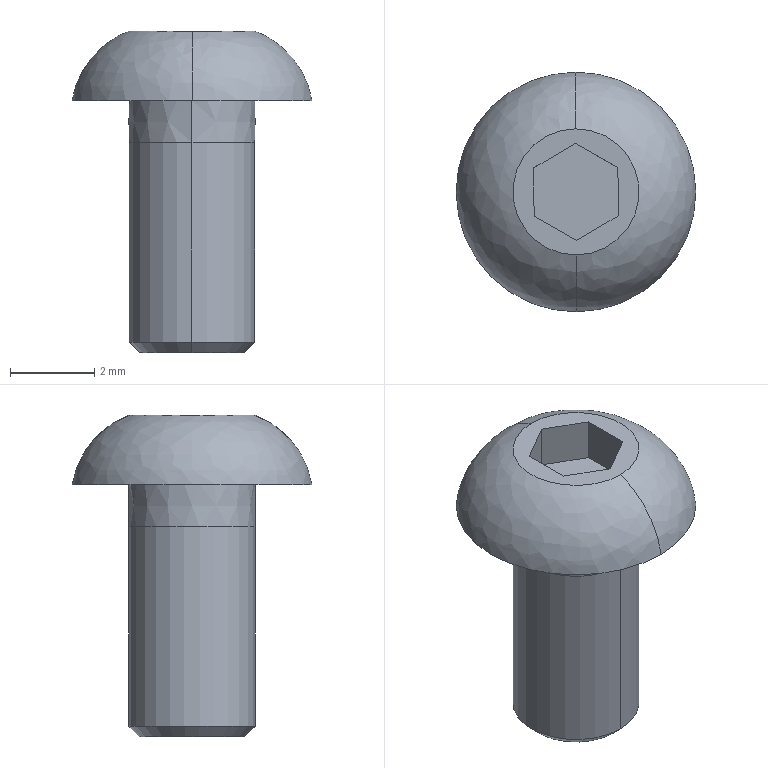Part | SolidWorks | features BaseBody 1 | 1 solid | 18 faces | box 5.7 x 5.7 x 7.65 mm | volume 69.708 mm3 | plane 10 | cone 4 | spline 2 | cylinder 2 | commonest cylinder face diameters 3 x2
STEP:
#1=CARTESIAN_POINT('',(555.46,-174.211,-71.234));
#2=VERTEX_POINT('',#1);
#3=CARTESIAN_POINT('',(555.435,-168.512,-71.234));
#4=VERTEX_POINT('',#3);
#5=CARTESIAN_POINT('',(555.447,-171.362,-71.234));
#6=DIRECTION('',(-0.000000001,0.000000003,-1.));
#7=DIRECTION('',(0.,1.,0.000000003));
#8=AXIS2_PLACEMENT_3D('',#5,#6,#7);
#9=CIRCLE('',#8,2.85);
#10=EDGE_CURVE('',#2,#4,#9,.T.);
#11=ORIENTED_EDGE('',*,*,#10,.F.);
#12=CARTESIAN_POINT('',(555.454,-172.861,-69.584));
#13=VERTEX_POINT('',#12);
#14=CARTESIAN_POINT('',(555.451,-172.111,-71.575));
#15=DIRECTION('',(-1.,-0.004352,0.000000001));
#16=DIRECTION('',(0.004352,-1.,-0.000000003));
#17=AXIS2_PLACEMENT_3D('',#14,#15,#16);
#18=CIRCLE('',#17,2.127);
#19=EDGE_CURVE('',#2,#13,#18,.T.);
#20=ORIENTED_EDGE('',*,*,#19,.T.);
#21=CARTESIAN_POINT('',(555.441,-169.862,-69.584));
#22=VERTEX_POINT('',#21);
#23=CARTESIAN_POINT('',(555.447,-171.362,-69.584));
#24=DIRECTION('',(-0.000000001,0.000000003,-1.));
#25=DIRECTION('',(0.,1.,0.000000003));
#26=AXIS2_PLACEMENT_3D('',#23,#24,#25);
#27=CIRCLE('',#26,1.5);
#28=EDGE_CURVE('',#13,#22,#27,.T.);
#29=ORIENTED_EDGE('',*,*,#28,.T.);
#30=CARTESIAN_POINT('',(555.444,-170.612,-71.575));
#31=DIRECTION('',(1.,0.004352,-0.000000001));
#32=DIRECTION('',(-0.004352,1.,0.000000003));
#33=AXIS2_PLACEMENT_3D('',#30,#31,#32);
#34=CIRCLE('',#33,2.127);
#35=EDGE_CURVE('',#4,#22,#34,.T.);
#36=ORIENTED_EDGE('',*,*,#35,.F.);
#37=EDGE_LOOP('',(#11,#20,#29,#36));
#38=FACE_OUTER_BOUND('',#37,.T.);
#39=CARTESIAN_POINT('',(555.46,-174.211,-71.234));
#40=CARTESIAN_POINT('',(549.76,-174.236,-71.234));
#41=CARTESIAN_POINT('',(549.735,-168.536,-71.234));
#42=CARTESIAN_POINT('',(555.435,-168.512,-71.234));
#43=CARTESIAN_POINT('',(555.459,-174.086,-70.464));
#44=CARTESIAN_POINT('',(550.009,-174.11,-70.464));
#45=CARTESIAN_POINT('',(549.986,-168.66,-70.464));
#46=CARTESIAN_POINT('',(555.436,-168.637,-70.464));
#47=CARTESIAN_POINT('',(555.457,-173.592,-69.859));
#48=CARTESIAN_POINT('',(550.996,-173.611,-69.859));
#49=CARTESIAN_POINT('',(550.977,-169.15,-69.859));
#50=CARTESIAN_POINT('',(555.438,-169.131,-69.859));
#51=CARTESIAN_POINT('',(555.454,-172.861,-69.584));
#52=CARTESIAN_POINT('',(552.454,-172.875,-69.584));
#53=CARTESIAN_POINT('',(552.441,-169.875,-69.584));
#54=CARTESIAN_POINT('',(555.441,-169.862,-69.584));
#55=(BOUNDED_SURFACE()B_SPLINE_SURFACE(3,3,((#39,#40,#41,#42),(#43,#44,#45,#46),(#47,#48,#49,#50),(#51,#52,#53,#54)),.UNSPECIFIED.,.F.,.F.,.T.)B_SPLINE_SURFACE_WITH_KNOTS((4,4),(4,4),(0.,1.),(0.,1.),.UNSPECIFIED.)GEOMETRIC_REPRESENTATION_ITEM()RATIONAL_B_SPLINE_SURFACE(((1.,0.3333,0.3333,1.),(0.9103,0.3034,0.3034,0.9103),(0.9103,0.3034,0.3034,0.9103),(1.,0.3333,0.3333,1.)))REPRESENTATION_ITEM('')SURFACE());
#56=ADVANCED_FACE('',(#38),#55,.T.);
#57=CARTESIAN_POINT('',(555.447,-169.862,-72.234));
#58=VERTEX_POINT('',#57);
#59=CARTESIAN_POINT('',(555.447,-172.862,-72.234));
#60=VERTEX_POINT('',#59);
#61=CARTESIAN_POINT('',(555.447,-171.362,-72.234));
#62=DIRECTION('',(-0.000000001,0.000000003,-1.));
#63=DIRECTION('',(0.,1.,0.000000003));
#64=AXIS2_PLACEMENT_3D('',#61,#62,#63);
#65=CIRCLE('',#64,1.5);
#66=EDGE_CURVE('',#58,#60,#65,.T.);
#67=ORIENTED_EDGE('',*,*,#66,.T.);
#68=CARTESIAN_POINT('',(555.447,-172.862,-76.984));
#69=VERTEX_POINT('',#68);
#70=CARTESIAN_POINT('',(555.447,-172.862,-74.609));
#71=DIRECTION('',(-0.000000001,0.000000003,-1.));
#72=VECTOR('',#71,1000.);
#73=LINE('',#70,#72);
#74=EDGE_CURVE('',#60,#69,#73,.T.);
#75=ORIENTED_EDGE('',*,*,#74,.T.);
#76=CARTESIAN_POINT('',(555.447,-169.862,-76.984));
#77=VERTEX_POINT('',#76);
#78=CARTESIAN_POINT('',(555.447,-171.362,-76.984));
#79=DIRECTION('',(0.000000001,-0.000000003,1.));
#80=DIRECTION('',(0.,1.,0.000000003));
#81=AXIS2_PLACEMENT_3D('',#78,#79,#80);
#82=CIRCLE('',#81,1.5);
#83=EDGE_CURVE('',#69,#77,#82,.T.);
#84=ORIENTED_EDGE('',*,*,#83,.T.);
#85=CARTESIAN_POINT('',(555.447,-169.862,-74.609));
#86=DIRECTION('',(-0.000000001,0.000000003,-1.));
#87=VECTOR('',#86,1000.);
#88=LINE('',#85,#87);
#89=EDGE_CURVE('',#58,#77,#88,.T.);
#90=ORIENTED_EDGE('',*,*,#89,.F.);
#91=EDGE_LOOP('',(#67,#75,#84,#90));
#92=FACE_OUTER_BOUND('',#91,.T.);
#93=CARTESIAN_POINT('',(555.447,-171.362,-74.609));
#94=DIRECTION('',(-0.000000001,0.000000003,-1.));
#95=DIRECTION('',(0.,1.,0.000000003));
#96=AXIS2_PLACEMENT_3D('',#93,#94,#95);
#97=CYLINDRICAL_SURFACE('',#96,1.5);
#98=ADVANCED_FACE('',(#92),#97,.T.);
#99=CARTESIAN_POINT('',(555.447,-172.612,-77.234));
#100=VERTEX_POINT('',#99);
#101=CARTESIAN_POINT('',(555.447,-170.112,-77.234));
#102=VERTEX_POINT('',#101);
#103=CARTESIAN_POINT('',(555.447,-171.362,-77.234));
#104=DIRECTION('',(0.000000001,-0.000000003,1.));
#105=DIRECTION('',(0.,-1.,-0.000000003));
#106=AXIS2_PLACEMENT_3D('',#103,#104,#105);
#107=CIRCLE('',#106,1.25);
#108=EDGE_CURVE('',#100,#102,#107,.T.);
#109=ORIENTED_EDGE('',*,*,#108,.T.);
#110=CARTESIAN_POINT('',(555.447,-169.862,-76.984));
#111=DIRECTION('',(0.000000001,0.7071,0.7071));
#112=VECTOR('',#111,1000.);
#113=LINE('',#110,#112);
#114=EDGE_CURVE('',#102,#77,#113,.T.);
#115=ORIENTED_EDGE('',*,*,#114,.T.);
#116=ORIENTED_EDGE('',*,*,#83,.F.);
#117=CARTESIAN_POINT('',(555.447,-172.862,-76.984));
#118=DIRECTION('',(0.000000001,-0.7071,0.7071));
#119=VECTOR('',#118,1000.);
#120=LINE('',#117,#119);
#121=EDGE_CURVE('',#100,#69,#120,.T.);
#122=ORIENTED_EDGE('',*,*,#121,.F.);
#123=EDGE_LOOP('',(#109,#115,#116,#122));
#124=FACE_OUTER_BOUND('',#123,.T.);
#125=CARTESIAN_POINT('',(555.447,-171.362,-76.984));
#126=DIRECTION('',(0.000000001,-0.000000003,1.));
#127=DIRECTION('',(0.,-1.,-0.000000003));
#128=AXIS2_PLACEMENT_3D('',#125,#126,#127);
#129=CONICAL_SURFACE('',#128,1.5,0.7854);
#130=ADVANCED_FACE('',(#124),#129,.T.);
#131=CARTESIAN_POINT('',(555.447,-169.862,-71.234));
#132=VERTEX_POINT('',#131);
#133=CARTESIAN_POINT('',(555.447,-172.861,-71.234));
#134=VERTEX_POINT('',#133);
#135=CARTESIAN_POINT('',(555.447,-171.362,-71.234));
#136=DIRECTION('',(-0.000000001,0.000000003,-1.));
#137=DIRECTION('',(0.,1.,0.000000003));
#138=AXIS2_PLACEMENT_3D('',#135,#136,#137);
#139=CIRCLE('',#138,1.499);
#140=EDGE_CURVE('',#132,#134,#139,.T.);
#141=ORIENTED_EDGE('',*,*,#140,.T.);
#142=CARTESIAN_POINT('',(555.447,-172.862,-72.234));
#143=DIRECTION('',(-0.000000001,-0.00075,-1.));
#144=VECTOR('',#143,1000.);
#145=LINE('',#142,#144);
#146=EDGE_CURVE('',#134,#60,#145,.T.);
#147=ORIENTED_EDGE('',*,*,#146,.T.);
#148=ORIENTED_EDGE('',*,*,#66,.F.);
#149=CARTESIAN_POINT('',(555.447,-169.862,-72.234));
#150=DIRECTION('',(-0.000000001,0.00075,-1.));
#151=VECTOR('',#150,1000.);
#152=LINE('',#149,#151);
#153=EDGE_CURVE('',#132,#58,#152,.T.);
#154=ORIENTED_EDGE('',*,*,#153,.F.);
#155=EDGE_LOOP('',(#141,#147,#148,#154));
#156=FACE_OUTER_BOUND('',#155,.T.);
#157=CARTESIAN_POINT('',(555.447,-171.362,-72.234));
#158=DIRECTION('',(-0.000000001,0.000000003,-1.));
#159=DIRECTION('',(0.,1.,0.000000003));
#160=AXIS2_PLACEMENT_3D('',#157,#158,#159);
#161=CONICAL_SURFACE('',#160,1.5,0.00075);
#162=ADVANCED_FACE('',(#156),#161,.T.);
#163=ORIENTED_EDGE('',*,*,#74,.F.);
#164=CARTESIAN_POINT('',(555.447,-171.362,-72.234));
#165=DIRECTION('',(-0.000000001,0.000000003,-1.));
#166=DIRECTION('',(0.,1.,0.000000003));
#167=AXIS2_PLACEMENT_3D('',#164,#165,#166);
#168=CIRCLE('',#167,1.5);
#169=EDGE_CURVE('',#60,#58,#168,.T.);
#170=ORIENTED_EDGE('',*,*,#169,.T.);
#171=ORIENTED_EDGE('',*,*,#89,.T.);
#172=CARTESIAN_POINT('',(555.447,-171.362,-76.984));
#173=DIRECTION('',(0.000000001,-0.000000003,1.));
#174=DIRECTION('',(0.,1.,0.000000003));
#175=AXIS2_PLACEMENT_3D('',#172,#173,#174);
#176=CIRCLE('',#175,1.5);
#177=EDGE_CURVE('',#77,#69,#176,.T.);
#178=ORIENTED_EDGE('',*,*,#177,.T.);
#179=EDGE_LOOP('',(#163,#170,#171,#178));
#180=FACE_OUTER_BOUND('',#179,.T.);
#181=CARTESIAN_POINT('',(555.447,-171.362,-74.609));
#182=DIRECTION('',(-0.000000001,0.000000003,-1.));
#183=DIRECTION('',(0.,1.,0.000000003));
#184=AXIS2_PLACEMENT_3D('',#181,#182,#183);
#185=CYLINDRICAL_SURFACE('',#184,1.5);
#186=ADVANCED_FACE('',(#180),#185,.T.);
#187=ORIENTED_EDGE('',*,*,#114,.F.);
#188=CARTESIAN_POINT('',(555.447,-171.362,-77.234));
#189=DIRECTION('',(0.000000001,-0.000000003,1.));
#190=DIRECTION('',(0.,-1.,-0.000000003));
#191=AXIS2_PLACEMENT_3D('',#188,#189,#190);
#192=CIRCLE('',#191,1.25);
#193=EDGE_CURVE('',#102,#100,#192,.T.);
#194=ORIENTED_EDGE('',*,*,#193,.T.);
#195=ORIENTED_EDGE('',*,*,#121,.T.);
#196=ORIENTED_EDGE('',*,*,#177,.F.);
#197=EDGE_LOOP('',(#187,#194,#195,#196));
#198=FACE_OUTER_BOUND('',#197,.T.);
#199=CARTESIAN_POINT('',(555.447,-171.362,-76.984));
#200=DIRECTION('',(0.000000001,-0.000000003,1.));
#201=DIRECTION('',(0.,-1.,-0.000000003));
#202=AXIS2_PLACEMENT_3D('',#199,#200,#201);
#203=CONICAL_SURFACE('',#202,1.5,0.7854);
#204=ADVANCED_FACE('',(#198),#203,.T.);
#205=ORIENTED_EDGE('',*,*,#146,.F.);
#206=CARTESIAN_POINT('',(555.447,-171.362,-71.234));
#207=DIRECTION('',(-0.000000001,0.000000003,-1.));
#208=DIRECTION('',(0.,1.,0.000000003));
#209=AXIS2_PLACEMENT_3D('',#206,#207,#208);
#210=CIRCLE('',#209,1.499);
#211=EDGE_CURVE('',#134,#132,#210,.T.);
#212=ORIENTED_EDGE('',*,*,#211,.T.);
#213=ORIENTED_EDGE('',*,*,#153,.T.);
#214=ORIENTED_EDGE('',*,*,#169,.F.);
#215=EDGE_LOOP('',(#205,#212,#213,#214));
#216=FACE_OUTER_BOUND('',#215,.T.);
#217=CARTESIAN_POINT('',(555.447,-171.362,-72.234));
#218=DIRECTION('',(-0.000000001,0.000000003,-1.));
#219=DIRECTION('',(0.,1.,0.000000003));
#220=AXIS2_PLACEMENT_3D('',#217,#218,#219);
#221=CONICAL_SURFACE('',#220,1.5,0.00075);
#222=ADVANCED_FACE('',(#216),#221,.T.);
#223=ORIENTED_EDGE('',*,*,#108,.F.);
#224=ORIENTED_EDGE('',*,*,#193,.F.);
#225=EDGE_LOOP('',(#223,#224));
#226=FACE_OUTER_BOUND('',#225,.T.);
#227=CARTESIAN_POINT('',(555.445,-170.737,-77.234));
#228=DIRECTION('',(-0.000000001,0.000000003,-1.));
#229=DIRECTION('',(0.,1.,0.000000003));
#230=AXIS2_PLACEMENT_3D('',#227,#228,#229);
#231=PLANE('',#230);
#232=ADVANCED_FACE('',(#226),#231,.T.);
#233=ORIENTED_EDGE('',*,*,#140,.F.);
#234=ORIENTED_EDGE('',*,*,#211,.F.);
#235=EDGE_LOOP('',(#233,#234));
#236=FACE_BOUND('',#235,.T.);
#237=CARTESIAN_POINT('',(555.447,-171.362,-71.234));
#238=DIRECTION('',(-0.000000001,0.000000003,-1.));
#239=DIRECTION('',(0.,1.,0.000000003));
#240=AXIS2_PLACEMENT_3D('',#237,#238,#239);
#241=CIRCLE('',#240,2.85);
#242=EDGE_CURVE('',#4,#2,#241,.T.);
#243=ORIENTED_EDGE('',*,*,#242,.T.);
#244=ORIENTED_EDGE('',*,*,#10,.T.);
#245=EDGE_LOOP('',(#243,#244));
#246=FACE_OUTER_BOUND('',#245,.T.);
#247=CARTESIAN_POINT('',(555.441,-169.937,-71.234));
#248=DIRECTION('',(-0.000000001,0.000000003,-1.));
#249=DIRECTION('',(0.,1.,0.000000003));
#250=AXIS2_PLACEMENT_3D('',#247,#248,#249);
#251=PLANE('',#250);
#252=ADVANCED_FACE('',(#236,#246),#251,.T.);
#253=ORIENTED_EDGE('',*,*,#19,.F.);
#254=ORIENTED_EDGE('',*,*,#242,.F.);
#255=ORIENTED_EDGE('',*,*,#35,.T.);
#256=CARTESIAN_POINT('',(555.447,-171.362,-69.584));
#257=DIRECTION('',(-0.000000001,0.000000003,-1.));
#258=DIRECTION('',(0.,1.,0.000000003));
#259=AXIS2_PLACEMENT_3D('',#256,#257,#258);
#260=CIRCLE('',#259,1.5);
#261=EDGE_CURVE('',#22,#13,#260,.T.);
#262=ORIENTED_EDGE('',*,*,#261,.T.);
#263=EDGE_LOOP('',(#253,#254,#255,#262));
#264=FACE_OUTER_BOUND('',#263,.T.);
#265=CARTESIAN_POINT('',(555.435,-168.512,-71.234));
#266=CARTESIAN_POINT('',(561.135,-168.487,-71.234));
#267=CARTESIAN_POINT('',(561.16,-174.187,-71.234));
#268=CARTESIAN_POINT('',(555.46,-174.211,-71.234));
#269=CARTESIAN_POINT('',(555.436,-168.637,-70.464));
#270=CARTESIAN_POINT('',(560.885,-168.613,-70.464));
#271=CARTESIAN_POINT('',(560.909,-174.063,-70.464));
#272=CARTESIAN_POINT('',(555.459,-174.086,-70.464));
#273=CARTESIAN_POINT('',(555.438,-169.131,-69.859));
#274=CARTESIAN_POINT('',(559.899,-169.112,-69.859));
#275=CARTESIAN_POINT('',(559.918,-173.573,-69.859));
#276=CARTESIAN_POINT('',(555.457,-173.592,-69.859));
#277=CARTESIAN_POINT('',(555.441,-169.862,-69.584));
#278=CARTESIAN_POINT('',(558.441,-169.848,-69.584));
#279=CARTESIAN_POINT('',(558.454,-172.848,-69.584));
#280=CARTESIAN_POINT('',(555.454,-172.861,-69.584));
#281=(BOUNDED_SURFACE()B_SPLINE_SURFACE(3,3,((#265,#266,#267,#268),(#269,#270,#271,#272),(#273,#274,#275,#276),(#277,#278,#279,#280)),.UNSPECIFIED.,.F.,.F.,.F.)B_SPLINE_SURFACE_WITH_KNOTS((4,4),(4,4),(0.,1.),(0.,1.),.UNSPECIFIED.)GEOMETRIC_REPRESENTATION_ITEM()RATIONAL_B_SPLINE_SURFACE(((1.,0.3333,0.3333,1.),(0.9103,0.3034,0.3034,0.9103),(0.9103,0.3034,0.3034,0.9103),(1.,0.3333,0.3333,1.)))REPRESENTATION_ITEM('')SURFACE());
#282=ADVANCED_FACE('',(#264),#281,.T.);
#283=ORIENTED_EDGE('',*,*,#261,.F.);
#284=ORIENTED_EDGE('',*,*,#28,.F.);
#285=EDGE_LOOP('',(#283,#284));
#286=FACE_OUTER_BOUND('',#285,.T.);
#287=CARTESIAN_POINT('',(556.45,-171.934,-69.584));
#288=VERTEX_POINT('',#287);
#289=CARTESIAN_POINT('',(555.452,-172.516,-69.584));
#290=VERTEX_POINT('',#289);
#291=CARTESIAN_POINT('',(556.45,-171.934,-69.584));
#292=DIRECTION('',(-0.8638,-0.5038,-0.000000001));
#293=VECTOR('',#292,1000.);
#294=LINE('',#291,#293);
#295=EDGE_CURVE('',#288,#290,#294,.T.);
#296=ORIENTED_EDGE('',*,*,#295,.T.);
#297=CARTESIAN_POINT('',(554.45,-171.943,-69.584));
#298=VERTEX_POINT('',#297);
#299=CARTESIAN_POINT('',(555.452,-172.516,-69.584));
#300=DIRECTION('',(-0.8682,0.4962,0.000000002));
#301=VECTOR('',#300,1000.);
#302=LINE('',#299,#301);
#303=EDGE_CURVE('',#290,#298,#302,.T.);
#304=ORIENTED_EDGE('',*,*,#303,.T.);
#305=CARTESIAN_POINT('',(554.445,-170.789,-69.584));
#306=VERTEX_POINT('',#305);
#307=CARTESIAN_POINT('',(554.45,-171.943,-69.584));
#308=DIRECTION('',(-0.004352,1.,0.000000003));
#309=VECTOR('',#308,1000.);
#310=LINE('',#307,#309);
#311=EDGE_CURVE('',#298,#306,#310,.T.);
#312=ORIENTED_EDGE('',*,*,#311,.T.);
#313=CARTESIAN_POINT('',(555.442,-170.207,-69.584));
#314=VERTEX_POINT('',#313);
#315=CARTESIAN_POINT('',(554.445,-170.789,-69.584));
#316=DIRECTION('',(0.8638,0.5038,0.000000001));
#317=VECTOR('',#316,1000.);
#318=LINE('',#315,#317);
#319=EDGE_CURVE('',#306,#314,#318,.T.);
#320=ORIENTED_EDGE('',*,*,#319,.T.);
#321=CARTESIAN_POINT('',(556.445,-170.78,-69.584));
#322=VERTEX_POINT('',#321);
#323=CARTESIAN_POINT('',(555.442,-170.207,-69.584));
#324=DIRECTION('',(0.8682,-0.4962,-0.000000002));
#325=VECTOR('',#324,1000.);
#326=LINE('',#323,#325);
#327=EDGE_CURVE('',#314,#322,#326,.T.);
#328=ORIENTED_EDGE('',*,*,#327,.T.);
#329=CARTESIAN_POINT('',(556.445,-170.78,-69.584));
#330=DIRECTION('',(0.004352,-1.,-0.000000003));
#331=VECTOR('',#330,1000.);
#332=LINE('',#329,#331);
#333=EDGE_CURVE('',#322,#288,#332,.T.);
#334=ORIENTED_EDGE('',*,*,#333,.T.);
#335=EDGE_LOOP('',(#296,#304,#312,#320,#328,#334));
#336=FACE_BOUND('',#335,.T.);
#337=CARTESIAN_POINT('',(555.444,-170.612,-69.584));
#338=DIRECTION('',(0.000000001,-0.000000003,1.));
#339=DIRECTION('',(0.,-1.,-0.000000003));
#340=AXIS2_PLACEMENT_3D('',#337,#338,#339);
#341=PLANE('',#340);
#342=ADVANCED_FACE('',(#286,#336),#341,.T.);
#343=CARTESIAN_POINT('',(554.45,-171.943,-70.624));
#344=VERTEX_POINT('',#343);
#345=CARTESIAN_POINT('',(554.45,-171.943,-69.584));
#346=DIRECTION('',(0.000000001,0.000000002,-1.));
#347=VECTOR('',#346,1000.);
#348=LINE('',#345,#347);
#349=EDGE_CURVE('',#298,#344,#348,.T.);
#350=ORIENTED_EDGE('',*,*,#349,.F.);
#351=ORIENTED_EDGE('',*,*,#303,.F.);
#352=CARTESIAN_POINT('',(555.452,-172.516,-70.624));
#353=VERTEX_POINT('',#352);
#354=CARTESIAN_POINT('',(555.452,-172.516,-69.584));
#355=DIRECTION('',(-0.000000001,-0.000000002,1.));
#356=VECTOR('',#355,1000.);
#357=LINE('',#354,#356);
#358=EDGE_CURVE('',#353,#290,#357,.T.);
#359=ORIENTED_EDGE('',*,*,#358,.F.);
#360=CARTESIAN_POINT('',(554.45,-171.943,-70.624));
#361=DIRECTION('',(0.8682,-0.4962,0.));
#362=VECTOR('',#361,1000.);
#363=LINE('',#360,#362);
#364=EDGE_CURVE('',#344,#353,#363,.T.);
#365=ORIENTED_EDGE('',*,*,#364,.F.);
#366=EDGE_LOOP('',(#350,#351,#359,#365));
#367=FACE_OUTER_BOUND('',#366,.T.);
#368=CARTESIAN_POINT('',(554.45,-171.943,-69.584));
#369=DIRECTION('',(-0.4962,-0.8682,-0.000000003));
#370=DIRECTION('',(0.8682,-0.4962,0.));
#371=AXIS2_PLACEMENT_3D('',#368,#369,#370);
#372=PLANE('',#371);
#373=ADVANCED_FACE('',(#367),#372,.F.);
#374=ORIENTED_EDGE('',*,*,#358,.T.);
#375=ORIENTED_EDGE('',*,*,#295,.F.);
#376=CARTESIAN_POINT('',(556.45,-171.934,-70.624));
#377=VERTEX_POINT('',#376);
#378=CARTESIAN_POINT('',(556.45,-171.934,-69.584));
#379=DIRECTION('',(0.000000002,-0.000000003,1.));
#380=VECTOR('',#379,1000.);
#381=LINE('',#378,#380);
#382=EDGE_CURVE('',#377,#288,#381,.T.);
#383=ORIENTED_EDGE('',*,*,#382,.F.);
#384=CARTESIAN_POINT('',(555.452,-172.516,-70.624));
#385=DIRECTION('',(0.8638,0.5038,0.));
#386=VECTOR('',#385,1000.);
#387=LINE('',#384,#386);
#388=EDGE_CURVE('',#353,#377,#387,.T.);
#389=ORIENTED_EDGE('',*,*,#388,.F.);
#390=EDGE_LOOP('',(#374,#375,#383,#389));
#391=FACE_OUTER_BOUND('',#390,.T.);
#392=CARTESIAN_POINT('',(555.452,-172.516,-69.584));
#393=DIRECTION('',(0.5038,-0.8638,-0.000000003));
#394=DIRECTION('',(0.8638,0.5038,0.));
#395=AXIS2_PLACEMENT_3D('',#392,#393,#394);
#396=PLANE('',#395);
#397=ADVANCED_FACE('',(#391),#396,.F.);
#398=ORIENTED_EDGE('',*,*,#382,.T.);
#399=ORIENTED_EDGE('',*,*,#333,.F.);
#400=CARTESIAN_POINT('',(556.445,-170.78,-70.624));
#401=VERTEX_POINT('',#400);
#402=CARTESIAN_POINT('',(556.445,-170.78,-69.584));
#403=DIRECTION('',(0.000000001,0.,1.));
#404=VECTOR('',#403,1000.);
#405=LINE('',#402,#404);
#406=EDGE_CURVE('',#401,#322,#405,.T.);
#407=ORIENTED_EDGE('',*,*,#406,.F.);
#408=CARTESIAN_POINT('',(556.45,-171.934,-70.624));
#409=DIRECTION('',(-0.004352,1.,0.));
#410=VECTOR('',#409,1000.);
#411=LINE('',#408,#410);
#412=EDGE_CURVE('',#377,#401,#411,.T.);
#413=ORIENTED_EDGE('',*,*,#412,.F.);
#414=EDGE_LOOP('',(#398,#399,#407,#413));
#415=FACE_OUTER_BOUND('',#414,.T.);
#416=CARTESIAN_POINT('',(556.45,-171.934,-69.584));
#417=DIRECTION('',(1.,0.004352,-0.000000001));
#418=DIRECTION('',(-0.004352,1.,0.));
#419=AXIS2_PLACEMENT_3D('',#416,#417,#418);
#420=PLANE('',#419);
#421=ADVANCED_FACE('',(#415),#420,.F.);
#422=ORIENTED_EDGE('',*,*,#406,.T.);
#423=ORIENTED_EDGE('',*,*,#327,.F.);
#424=CARTESIAN_POINT('',(555.442,-170.207,-70.624));
#425=VERTEX_POINT('',#424);
#426=CARTESIAN_POINT('',(555.442,-170.207,-69.584));
#427=DIRECTION('',(-0.000000001,-0.000000002,1.));
#428=VECTOR('',#427,1000.);
#429=LINE('',#426,#428);
#430=EDGE_CURVE('',#425,#314,#429,.T.);
#431=ORIENTED_EDGE('',*,*,#430,.F.);
#432=CARTESIAN_POINT('',(556.445,-170.78,-70.624));
#433=DIRECTION('',(-0.8682,0.4962,0.));
#434=VECTOR('',#433,1000.);
#435=LINE('',#432,#434);
#436=EDGE_CURVE('',#401,#425,#435,.T.);
#437=ORIENTED_EDGE('',*,*,#436,.F.);
#438=EDGE_LOOP('',(#422,#423,#431,#437));
#439=FACE_OUTER_BOUND('',#438,.T.);
#440=CARTESIAN_POINT('',(556.445,-170.78,-69.584));
#441=DIRECTION('',(0.4962,0.8682,0.000000003));
#442=DIRECTION('',(-0.8682,0.4962,0.));
#443=AXIS2_PLACEMENT_3D('',#440,#441,#442);
#444=PLANE('',#443);
#445=ADVANCED_FACE('',(#439),#444,.F.);
#446=ORIENTED_EDGE('',*,*,#430,.T.);
#447=ORIENTED_EDGE('',*,*,#319,.F.);
#448=CARTESIAN_POINT('',(554.445,-170.789,-70.624));
#449=VERTEX_POINT('',#448);
#450=CARTESIAN_POINT('',(554.445,-170.789,-69.584));
#451=DIRECTION('',(0.000000002,-0.000000003,1.));
#452=VECTOR('',#451,1000.);
#453=LINE('',#450,#452);
#454=EDGE_CURVE('',#449,#306,#453,.T.);
#455=ORIENTED_EDGE('',*,*,#454,.F.);
#456=CARTESIAN_POINT('',(555.442,-170.207,-70.624));
#457=DIRECTION('',(-0.8638,-0.5038,0.));
#458=VECTOR('',#457,1000.);
#459=LINE('',#456,#458);
#460=EDGE_CURVE('',#425,#449,#459,.T.);
#461=ORIENTED_EDGE('',*,*,#460,.F.);
#462=EDGE_LOOP('',(#446,#447,#455,#461));
#463=FACE_OUTER_BOUND('',#462,.T.);
#464=CARTESIAN_POINT('',(555.442,-170.207,-69.584));
#465=DIRECTION('',(-0.5038,0.8638,0.000000003));
#466=DIRECTION('',(-0.8638,-0.5038,0.));
#467=AXIS2_PLACEMENT_3D('',#464,#465,#466);
#468=PLANE('',#467);
#469=ADVANCED_FACE('',(#463),#468,.F.);
#470=ORIENTED_EDGE('',*,*,#454,.T.);
#471=ORIENTED_EDGE('',*,*,#311,.F.);
#472=ORIENTED_EDGE('',*,*,#349,.T.);
#473=CARTESIAN_POINT('',(554.445,-170.789,-70.624));
#474=DIRECTION('',(0.004352,-1.,0.));
#475=VECTOR('',#474,1000.);
#476=LINE('',#473,#475);
#477=EDGE_CURVE('',#449,#344,#476,.T.);
#478=ORIENTED_EDGE('',*,*,#477,.F.);
#479=EDGE_LOOP('',(#470,#471,#472,#478));
#480=FACE_OUTER_BOUND('',#479,.T.);
#481=CARTESIAN_POINT('',(554.445,-170.789,-69.584));
#482=DIRECTION('',(-1.,-0.004352,0.000000001));
#483=DIRECTION('',(0.004352,-1.,0.));
#484=AXIS2_PLACEMENT_3D('',#481,#482,#483);
#485=PLANE('',#484);
#486=ADVANCED_FACE('',(#480),#485,.F.);
#487=ORIENTED_EDGE('',*,*,#436,.T.);
#488=ORIENTED_EDGE('',*,*,#460,.T.);
#489=ORIENTED_EDGE('',*,*,#477,.T.);
#490=ORIENTED_EDGE('',*,*,#364,.T.);
#491=ORIENTED_EDGE('',*,*,#388,.T.);
#492=ORIENTED_EDGE('',*,*,#412,.T.);
#493=EDGE_LOOP('',(#487,#488,#489,#490,#491,#492));
#494=FACE_OUTER_BOUND('',#493,.T.);
#495=CARTESIAN_POINT('',(555.447,-171.362,-70.624));
#496=DIRECTION('',(0.000000001,-0.000000003,1.));
#497=DIRECTION('',(0.,-1.,-0.000000003));
#498=AXIS2_PLACEMENT_3D('',#495,#496,#497);
#499=PLANE('',#498);
#500=ADVANCED_FACE('',(#494),#499,.T.);
#501=CLOSED_SHELL('',(#56,#98,#130,#162,#186,#204,#222,#232,#252,#282,#342,#373,#397,#421,#445,#469,#486,#500));
#502=MANIFOLD_SOLID_BREP('',#501);
#503=CARTESIAN_POINT('',(0.,0.,0.));
#504=DIRECTION('',(0.,0.,1.));
#505=DIRECTION('',(1.,0.,0.));
#506=AXIS2_PLACEMENT_3D('',#503,#504,#505);
#507=(LENGTH_UNIT()NAMED_UNIT(*)SI_UNIT(.MILLI.,.METRE.));
#508=UNCERTAINTY_MEASURE_WITH_UNIT(LENGTH_MEASURE(0.00001),#507,'','');
#509=(NAMED_UNIT(*)PLANE_ANGLE_UNIT()SI_UNIT($,.RADIAN.));
#510=(NAMED_UNIT(*)SI_UNIT($,.STERADIAN.)SOLID_ANGLE_UNIT());
#511=(GEOMETRIC_REPRESENTATION_CONTEXT(3)GLOBAL_UNCERTAINTY_ASSIGNED_CONTEXT((#508))GLOBAL_UNIT_ASSIGNED_CONTEXT((#507,#509,#510))REPRESENTATION_CONTEXT('',''));
#512=ADVANCED_BREP_SHAPE_REPRESENTATION('',(#502,#506),#511);